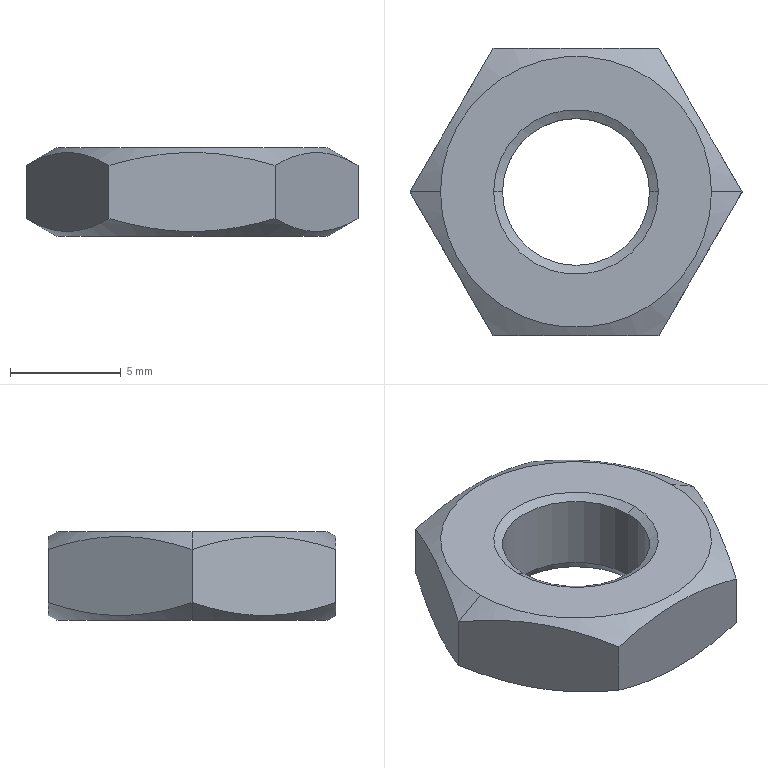Part | SolidWorks | features RevCut 2, Chamfer 1, Extrusion 1, LPattern 1 | 1 solid | 18 faces | box 15.011 x 13 x 4 mm | volume 430.713 mm3 | cone 8 | plane 8 | cylinder 2 | commonest cylinder face diameters 6.647 x2
STEP:
#1=CARTESIAN_POINT('',(-3.324,0.,-0.2309));
#2=VERTEX_POINT('',#1);
#3=CARTESIAN_POINT('',(3.324,0.,-0.2309));
#4=VERTEX_POINT('',#3);
#5=CARTESIAN_POINT('',(0.,0.,-0.2309));
#6=DIRECTION('',(0.,0.,1.));
#7=DIRECTION('',(1.,0.,0.));
#8=AXIS2_PLACEMENT_3D('',#5,#6,#7);
#9=CIRCLE('',#8,3.324);
#10=EDGE_CURVE('',#2,#4,#9,.T.);
#11=ORIENTED_EDGE('',*,*,#10,.F.);
#12=CARTESIAN_POINT('',(-3.724,0.,0.));
#13=VERTEX_POINT('',#12);
#14=CARTESIAN_POINT('',(-3.324,0.,-0.2309));
#15=DIRECTION('',(-0.866,0.,0.5));
#16=VECTOR('',#15,1000.);
#17=LINE('',#14,#16);
#18=EDGE_CURVE('',#2,#13,#17,.T.);
#19=ORIENTED_EDGE('',*,*,#18,.T.);
#20=CARTESIAN_POINT('',(3.724,0.,0.));
#21=VERTEX_POINT('',#20);
#22=CARTESIAN_POINT('',(0.,0.,0.));
#23=DIRECTION('',(0.,0.,-1.));
#24=DIRECTION('',(1.,0.,0.));
#25=AXIS2_PLACEMENT_3D('',#22,#23,#24);
#26=CIRCLE('',#25,3.724);
#27=EDGE_CURVE('',#21,#13,#26,.T.);
#28=ORIENTED_EDGE('',*,*,#27,.F.);
#29=CARTESIAN_POINT('',(3.324,0.,-0.2309));
#30=DIRECTION('',(0.866,0.,0.5));
#31=VECTOR('',#30,1000.);
#32=LINE('',#29,#31);
#33=EDGE_CURVE('',#4,#21,#32,.T.);
#34=ORIENTED_EDGE('',*,*,#33,.F.);
#35=EDGE_LOOP('',(#11,#19,#28,#34));
#36=FACE_OUTER_BOUND('',#35,.T.);
#37=CARTESIAN_POINT('',(0.,0.,-0.2309));
#38=DIRECTION('',(0.,0.,1.));
#39=DIRECTION('',(1.,0.,0.));
#40=AXIS2_PLACEMENT_3D('',#37,#38,#39);
#41=CONICAL_SURFACE('',#40,3.324,1.047);
#42=ADVANCED_FACE('',(#36),#41,.F.);
#43=CARTESIAN_POINT('',(3.324,0.,-3.6));
#44=VERTEX_POINT('',#43);
#45=CARTESIAN_POINT('',(-3.324,0.,-3.6));
#46=VERTEX_POINT('',#45);
#47=CARTESIAN_POINT('',(0.,0.,-3.6));
#48=DIRECTION('',(0.,0.,-1.));
#49=DIRECTION('',(1.,0.,0.));
#50=AXIS2_PLACEMENT_3D('',#47,#48,#49);
#51=CIRCLE('',#50,3.324);
#52=EDGE_CURVE('',#44,#46,#51,.T.);
#53=ORIENTED_EDGE('',*,*,#52,.F.);
#54=CARTESIAN_POINT('',(3.554,0.,-4.));
#55=VERTEX_POINT('',#54);
#56=CARTESIAN_POINT('',(3.554,0.,-4.));
#57=DIRECTION('',(0.5,0.,-0.866));
#58=VECTOR('',#57,1000.);
#59=LINE('',#56,#58);
#60=EDGE_CURVE('',#44,#55,#59,.T.);
#61=ORIENTED_EDGE('',*,*,#60,.T.);
#62=CARTESIAN_POINT('',(-3.554,0.,-4.));
#63=VERTEX_POINT('',#62);
#64=CARTESIAN_POINT('',(0.,0.,-4.));
#65=DIRECTION('',(0.,0.,1.));
#66=DIRECTION('',(1.,0.,0.));
#67=AXIS2_PLACEMENT_3D('',#64,#65,#66);
#68=CIRCLE('',#67,3.554);
#69=EDGE_CURVE('',#63,#55,#68,.T.);
#70=ORIENTED_EDGE('',*,*,#69,.F.);
#71=CARTESIAN_POINT('',(-3.554,0.,-4.));
#72=DIRECTION('',(-0.5,0.,-0.866));
#73=VECTOR('',#72,1000.);
#74=LINE('',#71,#73);
#75=EDGE_CURVE('',#46,#63,#74,.T.);
#76=ORIENTED_EDGE('',*,*,#75,.F.);
#77=EDGE_LOOP('',(#53,#61,#70,#76));
#78=FACE_OUTER_BOUND('',#77,.T.);
#79=CARTESIAN_POINT('',(0.,0.,-4.));
#80=DIRECTION('',(0.,0.,-1.));
#81=DIRECTION('',(-1.,0.,0.));
#82=AXIS2_PLACEMENT_3D('',#79,#80,#81);
#83=CONICAL_SURFACE('',#82,3.554,0.5236);
#84=ADVANCED_FACE('',(#78),#83,.F.);
#85=CARTESIAN_POINT('',(-6.125,0.,0.));
#86=VERTEX_POINT('',#85);
#87=CARTESIAN_POINT('',(6.125,0.,0.));
#88=VERTEX_POINT('',#87);
#89=CARTESIAN_POINT('',(0.,0.,0.));
#90=DIRECTION('',(0.,0.,-1.));
#91=DIRECTION('',(-1.,0.,0.));
#92=AXIS2_PLACEMENT_3D('',#89,#90,#91);
#93=CIRCLE('',#92,6.125);
#94=EDGE_CURVE('',#86,#88,#93,.T.);
#95=ORIENTED_EDGE('',*,*,#94,.T.);
#96=CARTESIAN_POINT('',(7.506,0.,-0.7971));
#97=VERTEX_POINT('',#96);
#98=CARTESIAN_POINT('',(6.125,0.,0.));
#99=DIRECTION('',(0.866,0.,-0.5));
#100=VECTOR('',#99,1000.);
#101=LINE('',#98,#100);
#102=EDGE_CURVE('',#88,#97,#101,.T.);
#103=ORIENTED_EDGE('',*,*,#102,.T.);
#104=CARTESIAN_POINT('',(3.753,6.5,-0.7971));
#105=VERTEX_POINT('',#104);
#106=CARTESIAN_POINT('',(7.506,0.,-0.7971));
#107=CARTESIAN_POINT('',(7.199,0.5307,-0.6202));
#108=CARTESIAN_POINT('',(6.891,1.065,-0.4744));
#109=CARTESIAN_POINT('',(6.267,2.145,-0.2724));
#110=CARTESIAN_POINT('',(5.952,2.691,-0.2169));
#111=CARTESIAN_POINT('',(5.473,3.52,-0.2163));
#112=CARTESIAN_POINT('',(5.313,3.798,-0.2299));
#113=CARTESIAN_POINT('',(4.996,4.347,-0.2828));
#114=CARTESIAN_POINT('',(4.838,4.62,-0.3221));
#115=CARTESIAN_POINT('',(4.369,5.433,-0.4738));
#116=CARTESIAN_POINT('',(4.06,5.969,-0.62));
#117=CARTESIAN_POINT('',(3.753,6.5,-0.7971));
#118=B_SPLINE_CURVE_WITH_KNOTS('',3,(#106,#107,#108,#109,#110,#111,#112,#113,#114,#115,#116,#117),.UNSPECIFIED.,.F.,.F.,(4,2,2,2,2,4),(0.000000238,0.001895,0.00379,0.004738,0.005685,0.00758),.UNSPECIFIED.);
#119=EDGE_CURVE('',#97,#105,#118,.T.);
#120=ORIENTED_EDGE('',*,*,#119,.T.);
#121=CARTESIAN_POINT('',(-3.753,6.5,-0.7971));
#122=VERTEX_POINT('',#121);
#123=CARTESIAN_POINT('',(3.753,6.5,-0.7971));
#124=CARTESIAN_POINT('',(3.146,6.5,-0.6219));
#125=CARTESIAN_POINT('',(2.532,6.5,-0.4761));
#126=CARTESIAN_POINT('',(1.278,6.5,-0.2726));
#127=CARTESIAN_POINT('',(0.6353,6.5,-0.2166));
#128=CARTESIAN_POINT('',(-0.6332,6.5,-0.2164));
#129=CARTESIAN_POINT('',(-1.263,6.5,-0.2709));
#130=CARTESIAN_POINT('',(-2.517,6.5,-0.473));
#131=CARTESIAN_POINT('',(-3.142,6.5,-0.6208));
#132=CARTESIAN_POINT('',(-3.753,6.5,-0.7971));
#133=B_SPLINE_CURVE_WITH_KNOTS('',3,(#123,#124,#125,#126,#127,#128,#129,#130,#131,#132),.UNSPECIFIED.,.F.,.F.,(4,2,2,2,4),(0.002787,0.004681,0.006575,0.008469,0.01036),.UNSPECIFIED.);
#134=EDGE_CURVE('',#105,#122,#133,.T.);
#135=ORIENTED_EDGE('',*,*,#134,.T.);
#136=CARTESIAN_POINT('',(-7.506,0.,-0.7971));
#137=VERTEX_POINT('',#136);
#138=CARTESIAN_POINT('',(-3.753,6.5,-0.7971));
#139=CARTESIAN_POINT('',(-4.059,5.969,-0.6202));
#140=CARTESIAN_POINT('',(-4.368,5.435,-0.4744));
#141=CARTESIAN_POINT('',(-4.991,4.355,-0.2724));
#142=CARTESIAN_POINT('',(-5.307,3.809,-0.2169));
#143=CARTESIAN_POINT('',(-5.785,2.98,-0.2163));
#144=CARTESIAN_POINT('',(-5.945,2.702,-0.2299));
#145=CARTESIAN_POINT('',(-6.262,2.153,-0.2828));
#146=CARTESIAN_POINT('',(-6.42,1.88,-0.3221));
#147=CARTESIAN_POINT('',(-6.889,1.067,-0.4738));
#148=CARTESIAN_POINT('',(-7.199,0.5313,-0.62));
#149=CARTESIAN_POINT('',(-7.506,0.,-0.7971));
#150=B_SPLINE_CURVE_WITH_KNOTS('',3,(#138,#139,#140,#141,#142,#143,#144,#145,#146,#147,#148,#149),.UNSPECIFIED.,.F.,.F.,(4,2,2,2,2,4),(0.000000238,0.001895,0.00379,0.004738,0.005685,0.00758),.UNSPECIFIED.);
#151=EDGE_CURVE('',#122,#137,#150,.T.);
#152=ORIENTED_EDGE('',*,*,#151,.T.);
#153=CARTESIAN_POINT('',(-6.125,0.,0.));
#154=DIRECTION('',(-0.866,0.,-0.5));
#155=VECTOR('',#154,1000.);
#156=LINE('',#153,#155);
#157=EDGE_CURVE('',#86,#137,#156,.T.);
#158=ORIENTED_EDGE('',*,*,#157,.F.);
#159=EDGE_LOOP('',(#95,#103,#120,#135,#152,#158));
#160=FACE_OUTER_BOUND('',#159,.T.);
#161=CARTESIAN_POINT('',(0.,0.,0.));
#162=DIRECTION('',(0.,0.,-1.));
#163=DIRECTION('',(-1.,0.,0.));
#164=AXIS2_PLACEMENT_3D('',#161,#162,#163);
#165=CONICAL_SURFACE('',#164,6.125,1.047);
#166=ADVANCED_FACE('',(#160),#165,.T.);
#167=CARTESIAN_POINT('',(-6.125,0.,-4.));
#168=VERTEX_POINT('',#167);
#169=CARTESIAN_POINT('',(6.125,0.,-4.));
#170=VERTEX_POINT('',#169);
#171=CARTESIAN_POINT('',(0.,0.,-4.));
#172=DIRECTION('',(0.,0.,-1.));
#173=DIRECTION('',(-1.,0.,0.));
#174=AXIS2_PLACEMENT_3D('',#171,#172,#173);
#175=CIRCLE('',#174,6.125);
#176=EDGE_CURVE('',#168,#170,#175,.T.);
#177=ORIENTED_EDGE('',*,*,#176,.F.);
#178=CARTESIAN_POINT('',(-7.506,0.,-3.203));
#179=VERTEX_POINT('',#178);
#180=CARTESIAN_POINT('',(-7.506,0.,-3.203));
#181=DIRECTION('',(-0.866,0.,0.5));
#182=VECTOR('',#181,1000.);
#183=LINE('',#180,#182);
#184=EDGE_CURVE('',#168,#179,#183,.T.);
#185=ORIENTED_EDGE('',*,*,#184,.T.);
#186=CARTESIAN_POINT('',(-3.753,6.5,-3.203));
#187=VERTEX_POINT('',#186);
#188=CARTESIAN_POINT('',(-7.506,0.,-3.203));
#189=CARTESIAN_POINT('',(-7.199,0.5307,-3.38));
#190=CARTESIAN_POINT('',(-6.891,1.065,-3.526));
#191=CARTESIAN_POINT('',(-6.267,2.145,-3.728));
#192=CARTESIAN_POINT('',(-5.952,2.691,-3.783));
#193=CARTESIAN_POINT('',(-5.473,3.52,-3.784));
#194=CARTESIAN_POINT('',(-5.313,3.798,-3.77));
#195=CARTESIAN_POINT('',(-4.996,4.347,-3.717));
#196=CARTESIAN_POINT('',(-4.838,4.62,-3.678));
#197=CARTESIAN_POINT('',(-4.369,5.433,-3.526));
#198=CARTESIAN_POINT('',(-4.06,5.969,-3.38));
#199=CARTESIAN_POINT('',(-3.753,6.5,-3.203));
#200=B_SPLINE_CURVE_WITH_KNOTS('',3,(#188,#189,#190,#191,#192,#193,#194,#195,#196,#197,#198,#199),.UNSPECIFIED.,.F.,.F.,(4,2,2,2,2,4),(0.000000238,0.001895,0.00379,0.004738,0.005685,0.00758),.UNSPECIFIED.);
#201=EDGE_CURVE('',#179,#187,#200,.T.);
#202=ORIENTED_EDGE('',*,*,#201,.T.);
#203=CARTESIAN_POINT('',(3.753,6.5,-3.203));
#204=VERTEX_POINT('',#203);
#205=CARTESIAN_POINT('',(-3.753,6.5,-3.203));
#206=CARTESIAN_POINT('',(-3.142,6.5,-3.379));
#207=CARTESIAN_POINT('',(-2.517,6.5,-3.527));
#208=CARTESIAN_POINT('',(-1.263,6.5,-3.729));
#209=CARTESIAN_POINT('',(-0.6332,6.5,-3.784));
#210=CARTESIAN_POINT('',(0.6353,6.5,-3.783));
#211=CARTESIAN_POINT('',(1.278,6.5,-3.727));
#212=CARTESIAN_POINT('',(2.532,6.5,-3.524));
#213=CARTESIAN_POINT('',(3.146,6.5,-3.378));
#214=CARTESIAN_POINT('',(3.753,6.5,-3.203));
#215=B_SPLINE_CURVE_WITH_KNOTS('',3,(#205,#206,#207,#208,#209,#210,#211,#212,#213,#214),.UNSPECIFIED.,.F.,.F.,(4,2,2,2,4),(0.006662,0.008561,0.01046,0.01236,0.01426),.UNSPECIFIED.);
#216=EDGE_CURVE('',#187,#204,#215,.T.);
#217=ORIENTED_EDGE('',*,*,#216,.T.);
#218=CARTESIAN_POINT('',(7.506,0.,-3.203));
#219=VERTEX_POINT('',#218);
#220=CARTESIAN_POINT('',(3.753,6.5,-3.203));
#221=CARTESIAN_POINT('',(4.059,5.969,-3.38));
#222=CARTESIAN_POINT('',(4.368,5.435,-3.526));
#223=CARTESIAN_POINT('',(4.991,4.355,-3.728));
#224=CARTESIAN_POINT('',(5.307,3.809,-3.783));
#225=CARTESIAN_POINT('',(5.785,2.98,-3.784));
#226=CARTESIAN_POINT('',(5.945,2.702,-3.77));
#227=CARTESIAN_POINT('',(6.262,2.153,-3.717));
#228=CARTESIAN_POINT('',(6.42,1.88,-3.678));
#229=CARTESIAN_POINT('',(6.889,1.067,-3.526));
#230=CARTESIAN_POINT('',(7.199,0.5313,-3.38));
#231=CARTESIAN_POINT('',(7.506,0.,-3.203));
#232=B_SPLINE_CURVE_WITH_KNOTS('',3,(#220,#221,#222,#223,#224,#225,#226,#227,#228,#229,#230,#231),.UNSPECIFIED.,.F.,.F.,(4,2,2,2,2,4),(0.000000238,0.001895,0.00379,0.004738,0.005685,0.00758),.UNSPECIFIED.);
#233=EDGE_CURVE('',#204,#219,#232,.T.);
#234=ORIENTED_EDGE('',*,*,#233,.T.);
#235=CARTESIAN_POINT('',(7.506,0.,-3.203));
#236=DIRECTION('',(0.866,0.,0.5));
#237=VECTOR('',#236,1000.);
#238=LINE('',#235,#237);
#239=EDGE_CURVE('',#170,#219,#238,.T.);
#240=ORIENTED_EDGE('',*,*,#239,.F.);
#241=EDGE_LOOP('',(#177,#185,#202,#217,#234,#240));
#242=FACE_OUTER_BOUND('',#241,.T.);
#243=CARTESIAN_POINT('',(0.,0.,-3.203));
#244=DIRECTION('',(0.,0.,1.));
#245=DIRECTION('',(1.,0.,0.));
#246=AXIS2_PLACEMENT_3D('',#243,#244,#245);
#247=CONICAL_SURFACE('',#246,7.506,1.047);
#248=ADVANCED_FACE('',(#242),#247,.T.);
#249=ORIENTED_EDGE('',*,*,#52,.T.);
#250=CARTESIAN_POINT('',(-3.324,0.,-4.));
#251=DIRECTION('',(0.,0.,1.));
#252=VECTOR('',#251,1000.);
#253=LINE('',#250,#252);
#254=EDGE_CURVE('',#46,#2,#253,.T.);
#255=ORIENTED_EDGE('',*,*,#254,.T.);
#256=ORIENTED_EDGE('',*,*,#10,.T.);
#257=CARTESIAN_POINT('',(3.324,0.,-4.));
#258=DIRECTION('',(0.,0.,1.));
#259=VECTOR('',#258,1000.);
#260=LINE('',#257,#259);
#261=EDGE_CURVE('',#44,#4,#260,.T.);
#262=ORIENTED_EDGE('',*,*,#261,.F.);
#263=EDGE_LOOP('',(#249,#255,#256,#262));
#264=FACE_OUTER_BOUND('',#263,.T.);
#265=CARTESIAN_POINT('',(0.,0.,-4.));
#266=DIRECTION('',(0.,0.,1.));
#267=DIRECTION('',(1.,0.,0.));
#268=AXIS2_PLACEMENT_3D('',#265,#266,#267);
#269=CYLINDRICAL_SURFACE('',#268,3.324);
#270=ADVANCED_FACE('',(#264),#269,.F.);
#271=CARTESIAN_POINT('',(-3.753,-6.5,-0.7971));
#272=VERTEX_POINT('',#271);
#273=CARTESIAN_POINT('',(3.753,-6.5,-0.7971));
#274=VERTEX_POINT('',#273);
#275=CARTESIAN_POINT('',(-3.753,-6.5,-0.7971));
#276=CARTESIAN_POINT('',(-3.142,-6.5,-0.6208));
#277=CARTESIAN_POINT('',(-2.517,-6.5,-0.473));
#278=CARTESIAN_POINT('',(-1.263,-6.5,-0.2709));
#279=CARTESIAN_POINT('',(-0.6332,-6.5,-0.2164));
#280=CARTESIAN_POINT('',(0.6353,-6.5,-0.2166));
#281=CARTESIAN_POINT('',(1.278,-6.5,-0.2726));
#282=CARTESIAN_POINT('',(2.532,-6.5,-0.4761));
#283=CARTESIAN_POINT('',(3.146,-6.5,-0.6219));
#284=CARTESIAN_POINT('',(3.753,-6.5,-0.7971));
#285=B_SPLINE_CURVE_WITH_KNOTS('',3,(#275,#276,#277,#278,#279,#280,#281,#282,#283,#284),.UNSPECIFIED.,.F.,.F.,(4,2,2,2,4),(0.006662,0.008561,0.01046,0.01236,0.01426),.UNSPECIFIED.);
#286=EDGE_CURVE('',#272,#274,#285,.T.);
#287=ORIENTED_EDGE('',*,*,#286,.F.);
#288=CARTESIAN_POINT('',(-3.753,-6.5,-3.203));
#289=VERTEX_POINT('',#288);
#290=CARTESIAN_POINT('',(-3.753,-6.5,-4.));
#291=DIRECTION('',(0.,0.,1.));
#292=VECTOR('',#291,1000.);
#293=LINE('',#290,#292);
#294=EDGE_CURVE('',#289,#272,#293,.T.);
#295=ORIENTED_EDGE('',*,*,#294,.F.);
#296=CARTESIAN_POINT('',(3.753,-6.5,-3.203));
#297=VERTEX_POINT('',#296);
#298=CARTESIAN_POINT('',(3.753,-6.5,-3.203));
#299=CARTESIAN_POINT('',(3.146,-6.5,-3.378));
#300=CARTESIAN_POINT('',(2.532,-6.5,-3.524));
#301=CARTESIAN_POINT('',(1.278,-6.5,-3.727));
#302=CARTESIAN_POINT('',(0.6353,-6.5,-3.783));
#303=CARTESIAN_POINT('',(-0.6332,-6.5,-3.784));
#304=CARTESIAN_POINT('',(-1.263,-6.5,-3.729));
#305=CARTESIAN_POINT('',(-2.517,-6.5,-3.527));
#306=CARTESIAN_POINT('',(-3.142,-6.5,-3.379));
#307=CARTESIAN_POINT('',(-3.753,-6.5,-3.203));
#308=B_SPLINE_CURVE_WITH_KNOTS('',3,(#298,#299,#300,#301,#302,#303,#304,#305,#306,#307),.UNSPECIFIED.,.F.,.F.,(4,2,2,2,4),(0.002787,0.004681,0.006575,0.008469,0.01036),.UNSPECIFIED.);
#309=EDGE_CURVE('',#297,#289,#308,.T.);
#310=ORIENTED_EDGE('',*,*,#309,.F.);
#311=CARTESIAN_POINT('',(3.753,-6.5,-4.));
#312=DIRECTION('',(0.,0.,1.));
#313=VECTOR('',#312,1000.);
#314=LINE('',#311,#313);
#315=EDGE_CURVE('',#297,#274,#314,.T.);
#316=ORIENTED_EDGE('',*,*,#315,.T.);
#317=EDGE_LOOP('',(#287,#295,#310,#316));
#318=FACE_OUTER_BOUND('',#317,.T.);
#319=CARTESIAN_POINT('',(-3.753,-6.5,-4.));
#320=DIRECTION('',(0.,-1.,0.));
#321=DIRECTION('',(1.,0.,0.));
#322=AXIS2_PLACEMENT_3D('',#319,#320,#321);
#323=PLANE('',#322);
#324=ADVANCED_FACE('',(#318),#323,.T.);
#325=CARTESIAN_POINT('',(-7.506,0.,-0.7971));
#326=CARTESIAN_POINT('',(-7.199,-0.5307,-0.6202));
#327=CARTESIAN_POINT('',(-6.891,-1.065,-0.4744));
#328=CARTESIAN_POINT('',(-6.267,-2.145,-0.2724));
#329=CARTESIAN_POINT('',(-5.952,-2.691,-0.2169));
#330=CARTESIAN_POINT('',(-5.473,-3.52,-0.2163));
#331=CARTESIAN_POINT('',(-5.313,-3.798,-0.2299));
#332=CARTESIAN_POINT('',(-4.996,-4.347,-0.2828));
#333=CARTESIAN_POINT('',(-4.838,-4.62,-0.3221));
#334=CARTESIAN_POINT('',(-4.369,-5.433,-0.4738));
#335=CARTESIAN_POINT('',(-4.06,-5.969,-0.62));
#336=CARTESIAN_POINT('',(-3.753,-6.5,-0.7971));
#337=B_SPLINE_CURVE_WITH_KNOTS('',3,(#325,#326,#327,#328,#329,#330,#331,#332,#333,#334,#335,#336),.UNSPECIFIED.,.F.,.F.,(4,2,2,2,2,4),(0.000000238,0.001895,0.00379,0.004738,0.005685,0.00758),.UNSPECIFIED.);
#338=EDGE_CURVE('',#137,#272,#337,.T.);
#339=ORIENTED_EDGE('',*,*,#338,.F.);
#340=CARTESIAN_POINT('',(-7.506,0.,-4.));
#341=DIRECTION('',(0.,0.,1.));
#342=VECTOR('',#341,1000.);
#343=LINE('',#340,#342);
#344=EDGE_CURVE('',#179,#137,#343,.T.);
#345=ORIENTED_EDGE('',*,*,#344,.F.);
#346=CARTESIAN_POINT('',(-3.753,-6.5,-3.203));
#347=CARTESIAN_POINT('',(-4.059,-5.969,-3.38));
#348=CARTESIAN_POINT('',(-4.368,-5.435,-3.526));
#349=CARTESIAN_POINT('',(-4.991,-4.355,-3.728));
#350=CARTESIAN_POINT('',(-5.307,-3.809,-3.783));
#351=CARTESIAN_POINT('',(-5.785,-2.98,-3.784));
#352=CARTESIAN_POINT('',(-5.945,-2.702,-3.77));
#353=CARTESIAN_POINT('',(-6.262,-2.153,-3.717));
#354=CARTESIAN_POINT('',(-6.42,-1.88,-3.678));
#355=CARTESIAN_POINT('',(-6.889,-1.067,-3.526));
#356=CARTESIAN_POINT('',(-7.199,-0.5313,-3.38));
#357=CARTESIAN_POINT('',(-7.506,0.,-3.203));
#358=B_SPLINE_CURVE_WITH_KNOTS('',3,(#346,#347,#348,#349,#350,#351,#352,#353,#354,#355,#356,#357),.UNSPECIFIED.,.F.,.F.,(4,2,2,2,2,4),(0.000000238,0.001895,0.00379,0.004738,0.005685,0.00758),.UNSPECIFIED.);
#359=EDGE_CURVE('',#289,#179,#358,.T.);
#360=ORIENTED_EDGE('',*,*,#359,.F.);
#361=ORIENTED_EDGE('',*,*,#294,.T.);
#362=EDGE_LOOP('',(#339,#345,#360,#361));
#363=FACE_OUTER_BOUND('',#362,.T.);
#364=CARTESIAN_POINT('',(-7.506,0.,-4.));
#365=DIRECTION('',(-0.866,-0.5,0.));
#366=DIRECTION('',(0.5,-0.866,0.));
#367=AXIS2_PLACEMENT_3D('',#364,#365,#366);
#368=PLANE('',#367);
#369=ADVANCED_FACE('',(#363),#368,.T.);
#370=ORIENTED_EDGE('',*,*,#151,.F.);
#371=CARTESIAN_POINT('',(-3.753,6.5,-4.));
#372=DIRECTION('',(0.,0.,1.));
#373=VECTOR('',#372,1000.);
#374=LINE('',#371,#373);
#375=EDGE_CURVE('',#187,#122,#374,.T.);
#376=ORIENTED_EDGE('',*,*,#375,.F.);
#377=ORIENTED_EDGE('',*,*,#201,.F.);
#378=ORIENTED_EDGE('',*,*,#344,.T.);
#379=EDGE_LOOP('',(#370,#376,#377,#378));
#380=FACE_OUTER_BOUND('',#379,.T.);
#381=CARTESIAN_POINT('',(-3.753,6.5,-4.));
#382=DIRECTION('',(-0.866,0.5,0.));
#383=DIRECTION('',(-0.5,-0.866,0.));
#384=AXIS2_PLACEMENT_3D('',#381,#382,#383);
#385=PLANE('',#384);
#386=ADVANCED_FACE('',(#380),#385,.T.);
#387=ORIENTED_EDGE('',*,*,#134,.F.);
#388=CARTESIAN_POINT('',(3.753,6.5,-4.));
#389=DIRECTION('',(0.,0.,1.));
#390=VECTOR('',#389,1000.);
#391=LINE('',#388,#390);
#392=EDGE_CURVE('',#204,#105,#391,.T.);
#393=ORIENTED_EDGE('',*,*,#392,.F.);
#394=ORIENTED_EDGE('',*,*,#216,.F.);
#395=ORIENTED_EDGE('',*,*,#375,.T.);
#396=EDGE_LOOP('',(#387,#393,#394,#395));
#397=FACE_OUTER_BOUND('',#396,.T.);
#398=CARTESIAN_POINT('',(3.753,6.5,-4.));
#399=DIRECTION('',(0.,1.,0.));
#400=DIRECTION('',(0.,0.,1.));
#401=AXIS2_PLACEMENT_3D('',#398,#399,#400);
#402=PLANE('',#401);
#403=ADVANCED_FACE('',(#397),#402,.T.);
#404=ORIENTED_EDGE('',*,*,#119,.F.);
#405=CARTESIAN_POINT('',(7.506,0.,-4.));
#406=DIRECTION('',(0.,0.,1.));
#407=VECTOR('',#406,1000.);
#408=LINE('',#405,#407);
#409=EDGE_CURVE('',#219,#97,#408,.T.);
#410=ORIENTED_EDGE('',*,*,#409,.F.);
#411=ORIENTED_EDGE('',*,*,#233,.F.);
#412=ORIENTED_EDGE('',*,*,#392,.T.);
#413=EDGE_LOOP('',(#404,#410,#411,#412));
#414=FACE_OUTER_BOUND('',#413,.T.);
#415=CARTESIAN_POINT('',(7.506,0.,-4.));
#416=DIRECTION('',(0.866,0.5,0.));
#417=DIRECTION('',(-0.5,0.866,0.));
#418=AXIS2_PLACEMENT_3D('',#415,#416,#417);
#419=PLANE('',#418);
#420=ADVANCED_FACE('',(#414),#419,.T.);
#421=CARTESIAN_POINT('',(3.753,-6.5,-0.7971));
#422=CARTESIAN_POINT('',(4.059,-5.969,-0.6202));
#423=CARTESIAN_POINT('',(4.368,-5.435,-0.4744));
#424=CARTESIAN_POINT('',(4.991,-4.355,-0.2724));
#425=CARTESIAN_POINT('',(5.307,-3.809,-0.2169));
#426=CARTESIAN_POINT('',(5.785,-2.98,-0.2163));
#427=CARTESIAN_POINT('',(5.945,-2.702,-0.2299));
#428=CARTESIAN_POINT('',(6.262,-2.153,-0.2828));
#429=CARTESIAN_POINT('',(6.42,-1.88,-0.3221));
#430=CARTESIAN_POINT('',(6.889,-1.067,-0.4738));
#431=CARTESIAN_POINT('',(7.199,-0.5313,-0.62));
#432=CARTESIAN_POINT('',(7.506,0.,-0.7971));
#433=B_SPLINE_CURVE_WITH_KNOTS('',3,(#421,#422,#423,#424,#425,#426,#427,#428,#429,#430,#431,#432),.UNSPECIFIED.,.F.,.F.,(4,2,2,2,2,4),(0.000000238,0.001895,0.00379,0.004738,0.005685,0.00758),.UNSPECIFIED.);
#434=EDGE_CURVE('',#274,#97,#433,.T.);
#435=ORIENTED_EDGE('',*,*,#434,.F.);
#436=ORIENTED_EDGE('',*,*,#315,.F.);
#437=CARTESIAN_POINT('',(7.506,0.,-3.203));
#438=CARTESIAN_POINT('',(7.199,-0.5307,-3.38));
#439=CARTESIAN_POINT('',(6.891,-1.065,-3.526));
#440=CARTESIAN_POINT('',(6.267,-2.145,-3.728));
#441=CARTESIAN_POINT('',(5.952,-2.691,-3.783));
#442=CARTESIAN_POINT('',(5.473,-3.52,-3.784));
#443=CARTESIAN_POINT('',(5.313,-3.798,-3.77));
#444=CARTESIAN_POINT('',(4.996,-4.347,-3.717));
#445=CARTESIAN_POINT('',(4.838,-4.62,-3.678));
#446=CARTESIAN_POINT('',(4.369,-5.433,-3.526));
#447=CARTESIAN_POINT('',(4.06,-5.969,-3.38));
#448=CARTESIAN_POINT('',(3.753,-6.5,-3.203));
#449=B_SPLINE_CURVE_WITH_KNOTS('',3,(#437,#438,#439,#440,#441,#442,#443,#444,#445,#446,#447,#448),.UNSPECIFIED.,.F.,.F.,(4,2,2,2,2,4),(0.000000238,0.001895,0.00379,0.004738,0.005685,0.00758),.UNSPECIFIED.);
#450=EDGE_CURVE('',#219,#297,#449,.T.);
#451=ORIENTED_EDGE('',*,*,#450,.F.);
#452=ORIENTED_EDGE('',*,*,#409,.T.);
#453=EDGE_LOOP('',(#435,#436,#451,#452));
#454=FACE_OUTER_BOUND('',#453,.T.);
#455=CARTESIAN_POINT('',(3.753,-6.5,-4.));
#456=DIRECTION('',(0.866,-0.5,0.));
#457=DIRECTION('',(0.5,0.866,0.));
#458=AXIS2_PLACEMENT_3D('',#455,#456,#457);
#459=PLANE('',#458);
#460=ADVANCED_FACE('',(#454),#459,.T.);
#461=ORIENTED_EDGE('',*,*,#69,.T.);
#462=CARTESIAN_POINT('',(0.,0.,-4.));
#463=DIRECTION('',(0.,0.,1.));
#464=DIRECTION('',(1.,0.,0.));
#465=AXIS2_PLACEMENT_3D('',#462,#463,#464);
#466=CIRCLE('',#465,3.554);
#467=EDGE_CURVE('',#55,#63,#466,.T.);
#468=ORIENTED_EDGE('',*,*,#467,.T.);
#469=EDGE_LOOP('',(#461,#468));
#470=FACE_BOUND('',#469,.T.);
#471=CARTESIAN_POINT('',(0.,0.,-4.));
#472=DIRECTION('',(0.,0.,-1.));
#473=DIRECTION('',(-1.,0.,0.));
#474=AXIS2_PLACEMENT_3D('',#471,#472,#473);
#475=CIRCLE('',#474,6.125);
#476=EDGE_CURVE('',#170,#168,#475,.T.);
#477=ORIENTED_EDGE('',*,*,#476,.T.);
#478=ORIENTED_EDGE('',*,*,#176,.T.);
#479=EDGE_LOOP('',(#477,#478));
#480=FACE_OUTER_BOUND('',#479,.T.);
#481=CARTESIAN_POINT('',(3.753,-6.5,-4.));
#482=DIRECTION('',(0.,0.,1.));
#483=DIRECTION('',(1.,0.,0.));
#484=AXIS2_PLACEMENT_3D('',#481,#482,#483);
#485=PLANE('',#484);
#486=ADVANCED_FACE('',(#470,#480),#485,.F.);
#487=ORIENTED_EDGE('',*,*,#27,.T.);
#488=CARTESIAN_POINT('',(0.,0.,0.));
#489=DIRECTION('',(0.,0.,-1.));
#490=DIRECTION('',(1.,0.,0.));
#491=AXIS2_PLACEMENT_3D('',#488,#489,#490);
#492=CIRCLE('',#491,3.724);
#493=EDGE_CURVE('',#13,#21,#492,.T.);
#494=ORIENTED_EDGE('',*,*,#493,.T.);
#495=EDGE_LOOP('',(#487,#494));
#496=FACE_BOUND('',#495,.T.);
#497=ORIENTED_EDGE('',*,*,#94,.F.);
#498=CARTESIAN_POINT('',(0.,0.,0.));
#499=DIRECTION('',(0.,0.,-1.));
#500=DIRECTION('',(-1.,0.,0.));
#501=AXIS2_PLACEMENT_3D('',#498,#499,#500);
#502=CIRCLE('',#501,6.125);
#503=EDGE_CURVE('',#88,#86,#502,.T.);
#504=ORIENTED_EDGE('',*,*,#503,.F.);
#505=EDGE_LOOP('',(#497,#504));
#506=FACE_OUTER_BOUND('',#505,.T.);
#507=CARTESIAN_POINT('',(3.753,-6.5,0.));
#508=DIRECTION('',(0.,0.,1.));
#509=DIRECTION('',(1.,0.,0.));
#510=AXIS2_PLACEMENT_3D('',#507,#508,#509);
#511=PLANE('',#510);
#512=ADVANCED_FACE('',(#496,#506),#511,.T.);
#513=ORIENTED_EDGE('',*,*,#254,.F.);
#514=CARTESIAN_POINT('',(0.,0.,-3.6));
#515=DIRECTION('',(0.,0.,-1.));
#516=DIRECTION('',(1.,0.,0.));
#517=AXIS2_PLACEMENT_3D('',#514,#515,#516);
#518=CIRCLE('',#517,3.324);
#519=EDGE_CURVE('',#46,#44,#518,.T.);
#520=ORIENTED_EDGE('',*,*,#519,.T.);
#521=ORIENTED_EDGE('',*,*,#261,.T.);
#522=CARTESIAN_POINT('',(0.,0.,-0.2309));
#523=DIRECTION('',(0.,0.,1.));
#524=DIRECTION('',(1.,0.,0.));
#525=AXIS2_PLACEMENT_3D('',#522,#523,#524);
#526=CIRCLE('',#525,3.324);
#527=EDGE_CURVE('',#4,#2,#526,.T.);
#528=ORIENTED_EDGE('',*,*,#527,.T.);
#529=EDGE_LOOP('',(#513,#520,#521,#528));
#530=FACE_OUTER_BOUND('',#529,.T.);
#531=CARTESIAN_POINT('',(0.,0.,-4.));
#532=DIRECTION('',(0.,0.,1.));
#533=DIRECTION('',(1.,0.,0.));
#534=AXIS2_PLACEMENT_3D('',#531,#532,#533);
#535=CYLINDRICAL_SURFACE('',#534,3.324);
#536=ADVANCED_FACE('',(#530),#535,.F.);
#537=ORIENTED_EDGE('',*,*,#184,.F.);
#538=ORIENTED_EDGE('',*,*,#476,.F.);
#539=ORIENTED_EDGE('',*,*,#239,.T.);
#540=ORIENTED_EDGE('',*,*,#450,.T.);
#541=ORIENTED_EDGE('',*,*,#309,.T.);
#542=ORIENTED_EDGE('',*,*,#359,.T.);
#543=EDGE_LOOP('',(#537,#538,#539,#540,#541,#542));
#544=FACE_OUTER_BOUND('',#543,.T.);
#545=CARTESIAN_POINT('',(0.,0.,-3.203));
#546=DIRECTION('',(0.,0.,1.));
#547=DIRECTION('',(1.,0.,0.));
#548=AXIS2_PLACEMENT_3D('',#545,#546,#547);
#549=CONICAL_SURFACE('',#548,7.506,1.047);
#550=ADVANCED_FACE('',(#544),#549,.T.);
#551=ORIENTED_EDGE('',*,*,#102,.F.);
#552=ORIENTED_EDGE('',*,*,#503,.T.);
#553=ORIENTED_EDGE('',*,*,#157,.T.);
#554=ORIENTED_EDGE('',*,*,#338,.T.);
#555=ORIENTED_EDGE('',*,*,#286,.T.);
#556=ORIENTED_EDGE('',*,*,#434,.T.);
#557=EDGE_LOOP('',(#551,#552,#553,#554,#555,#556));
#558=FACE_OUTER_BOUND('',#557,.T.);
#559=CARTESIAN_POINT('',(0.,0.,0.));
#560=DIRECTION('',(0.,0.,-1.));
#561=DIRECTION('',(-1.,0.,0.));
#562=AXIS2_PLACEMENT_3D('',#559,#560,#561);
#563=CONICAL_SURFACE('',#562,6.125,1.047);
#564=ADVANCED_FACE('',(#558),#563,.T.);
#565=ORIENTED_EDGE('',*,*,#60,.F.);
#566=ORIENTED_EDGE('',*,*,#519,.F.);
#567=ORIENTED_EDGE('',*,*,#75,.T.);
#568=ORIENTED_EDGE('',*,*,#467,.F.);
#569=EDGE_LOOP('',(#565,#566,#567,#568));
#570=FACE_OUTER_BOUND('',#569,.T.);
#571=CARTESIAN_POINT('',(0.,0.,-4.));
#572=DIRECTION('',(0.,0.,-1.));
#573=DIRECTION('',(-1.,0.,0.));
#574=AXIS2_PLACEMENT_3D('',#571,#572,#573);
#575=CONICAL_SURFACE('',#574,3.554,0.5236);
#576=ADVANCED_FACE('',(#570),#575,.F.);
#577=ORIENTED_EDGE('',*,*,#18,.F.);
#578=ORIENTED_EDGE('',*,*,#527,.F.);
#579=ORIENTED_EDGE('',*,*,#33,.T.);
#580=ORIENTED_EDGE('',*,*,#493,.F.);
#581=EDGE_LOOP('',(#577,#578,#579,#580));
#582=FACE_OUTER_BOUND('',#581,.T.);
#583=CARTESIAN_POINT('',(0.,0.,-0.2309));
#584=DIRECTION('',(0.,0.,1.));
#585=DIRECTION('',(1.,0.,0.));
#586=AXIS2_PLACEMENT_3D('',#583,#584,#585);
#587=CONICAL_SURFACE('',#586,3.324,1.047);
#588=ADVANCED_FACE('',(#582),#587,.F.);
#589=CLOSED_SHELL('',(#42,#84,#166,#248,#270,#324,#369,#386,#403,#420,#460,#486,#512,#536,#550,#564,#576,#588));
#590=MANIFOLD_SOLID_BREP('',#589);
#591=CARTESIAN_POINT('',(0.,0.,0.));
#592=DIRECTION('',(0.,0.,1.));
#593=DIRECTION('',(1.,0.,0.));
#594=AXIS2_PLACEMENT_3D('',#591,#592,#593);
#595=(LENGTH_UNIT()NAMED_UNIT(*)SI_UNIT(.MILLI.,.METRE.));
#596=UNCERTAINTY_MEASURE_WITH_UNIT(LENGTH_MEASURE(0.00001),#595,'','');
#597=(NAMED_UNIT(*)PLANE_ANGLE_UNIT()SI_UNIT($,.RADIAN.));
#598=(NAMED_UNIT(*)SI_UNIT($,.STERADIAN.)SOLID_ANGLE_UNIT());
#599=(GEOMETRIC_REPRESENTATION_CONTEXT(3)GLOBAL_UNCERTAINTY_ASSIGNED_CONTEXT((#596))GLOBAL_UNIT_ASSIGNED_CONTEXT((#595,#597,#598))REPRESENTATION_CONTEXT('',''));
#600=ADVANCED_BREP_SHAPE_REPRESENTATION('',(#590,#594),#599);